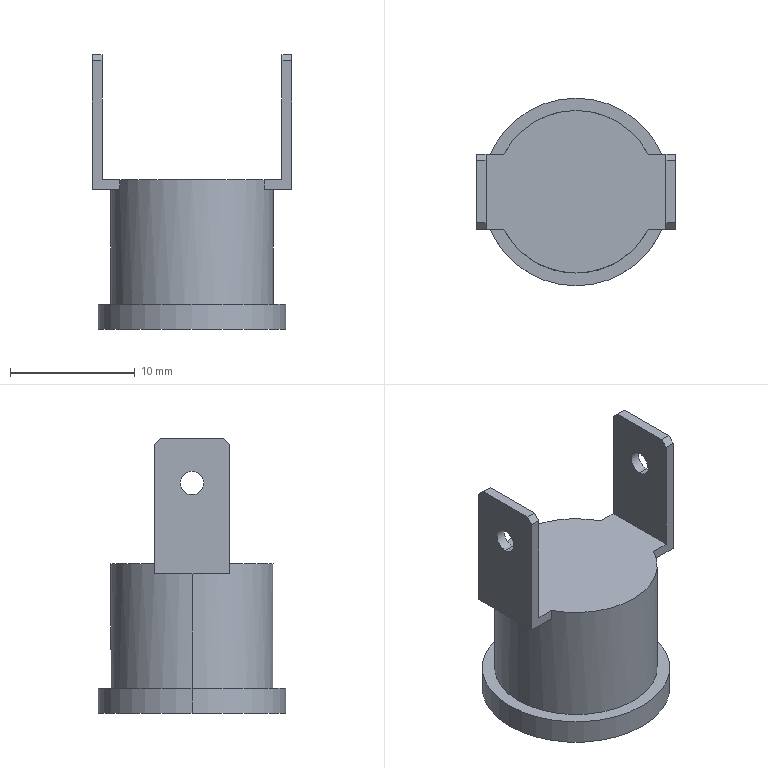Part | STEP file | WENKONG1_2_1_1_1 | 1 solid | 27 faces | box 16 x 15 x 22 mm | volume 1789 mm3 | plane 19 | cylinder 8 | commonest cylinder face diameters 1.882 x4 13 x2 15 x2
STEP:
#1=CARTESIAN_POINT('',(0.,0.,0.));
#2=DIRECTION('',(0.,0.,1.));
#3=DIRECTION('',(1.,0.,0.));
#4=AXIS2_PLACEMENT_3D('',#1,#2,#3);
#5=CARTESIAN_POINT('',(-8.,0.,19.375));
#6=VERTEX_POINT('',#5);
#7=CARTESIAN_POINT('',(-7.2,0.,19.375));
#8=VERTEX_POINT('',#7);
#9=CARTESIAN_POINT('',(-8.,0.,19.375));
#10=DIRECTION('',(1.,0.,0.));
#11=VECTOR('',#10,0.8);
#12=LINE('',#9,#11);
#13=EDGE_CURVE('',#6,#8,#12,.T.);
#14=ORIENTED_EDGE('',*,*,#13,.F.);
#15=CARTESIAN_POINT('',(-8.,0.,17.493));
#16=VERTEX_POINT('',#15);
#17=CARTESIAN_POINT('',(-8.,0.,18.434));
#18=DIRECTION('',(-1.,0.,0.));
#19=DIRECTION('',(0.,0.,-1.));
#20=AXIS2_PLACEMENT_3D('',#17,#18,#19);
#21=CIRCLE('',#20,0.941);
#22=EDGE_CURVE('',#16,#6,#21,.T.);
#23=ORIENTED_EDGE('',*,*,#22,.F.);
#24=CARTESIAN_POINT('',(-7.2,0.,17.493));
#25=VERTEX_POINT('',#24);
#26=CARTESIAN_POINT('',(-7.2,0.,17.493));
#27=DIRECTION('',(-1.,0.,0.));
#28=VECTOR('',#27,0.8);
#29=LINE('',#26,#28);
#30=EDGE_CURVE('',#25,#16,#29,.T.);
#31=ORIENTED_EDGE('',*,*,#30,.F.);
#32=CARTESIAN_POINT('',(-7.2,0.,18.434));
#33=DIRECTION('',(1.,0.,0.));
#34=DIRECTION('',(0.,0.,1.));
#35=AXIS2_PLACEMENT_3D('',#32,#33,#34);
#36=CIRCLE('',#35,0.941);
#37=EDGE_CURVE('',#8,#25,#36,.T.);
#38=ORIENTED_EDGE('',*,*,#37,.F.);
#39=EDGE_LOOP('',(#14,#23,#31,#38));
#40=FACE_OUTER_BOUND('',#39,.F.);
#41=CARTESIAN_POINT('',(-7.6,0.,18.434));
#42=DIRECTION('',(-1.,0.,0.));
#43=DIRECTION('',(0.,0.,-1.));
#44=AXIS2_PLACEMENT_3D('',#41,#42,#43);
#45=CYLINDRICAL_SURFACE('',#44,0.941);
#46=ADVANCED_FACE('',(#40),#45,.F.);
#47=CARTESIAN_POINT('',(-8.,0.,18.434));
#48=DIRECTION('',(-1.,0.,0.));
#49=DIRECTION('',(0.,0.,1.));
#50=AXIS2_PLACEMENT_3D('',#47,#48,#49);
#51=CIRCLE('',#50,0.941);
#52=EDGE_CURVE('',#6,#16,#51,.T.);
#53=ORIENTED_EDGE('',*,*,#52,.F.);
#54=ORIENTED_EDGE('',*,*,#13,.T.);
#55=CARTESIAN_POINT('',(-7.2,0.,18.434));
#56=DIRECTION('',(1.,0.,0.));
#57=DIRECTION('',(0.,0.,-1.));
#58=AXIS2_PLACEMENT_3D('',#55,#56,#57);
#59=CIRCLE('',#58,0.941);
#60=EDGE_CURVE('',#25,#8,#59,.T.);
#61=ORIENTED_EDGE('',*,*,#60,.F.);
#62=ORIENTED_EDGE('',*,*,#30,.T.);
#63=EDGE_LOOP('',(#53,#54,#61,#62));
#64=FACE_OUTER_BOUND('',#63,.F.);
#65=CARTESIAN_POINT('',(-7.6,0.,18.434));
#66=DIRECTION('',(-1.,0.,0.));
#67=DIRECTION('',(0.,0.,1.));
#68=AXIS2_PLACEMENT_3D('',#65,#66,#67);
#69=CYLINDRICAL_SURFACE('',#68,0.941);
#70=ADVANCED_FACE('',(#64),#69,.F.);
#71=CARTESIAN_POINT('',(-8.,2.5,22.));
#72=VERTEX_POINT('',#71);
#73=CARTESIAN_POINT('',(-8.,-2.5,22.));
#74=VERTEX_POINT('',#73);
#75=CARTESIAN_POINT('',(-8.,2.5,22.));
#76=DIRECTION('',(0.,-1.,0.));
#77=VECTOR('',#76,5.);
#78=LINE('',#75,#77);
#79=EDGE_CURVE('',#72,#74,#78,.T.);
#80=ORIENTED_EDGE('',*,*,#79,.T.);
#81=CARTESIAN_POINT('',(-8.,-3.,21.5));
#82=VERTEX_POINT('',#81);
#83=CARTESIAN_POINT('',(-8.,-2.5,22.));
#84=DIRECTION('',(0.,-0.7071,-0.7071));
#85=VECTOR('',#84,0.7071);
#86=LINE('',#83,#85);
#87=EDGE_CURVE('',#74,#82,#86,.T.);
#88=ORIENTED_EDGE('',*,*,#87,.T.);
#89=CARTESIAN_POINT('',(-8.,-3.,11.2));
#90=VERTEX_POINT('',#89);
#91=CARTESIAN_POINT('',(-8.,-3.,21.5));
#92=DIRECTION('',(0.,0.,-1.));
#93=VECTOR('',#92,10.3);
#94=LINE('',#91,#93);
#95=EDGE_CURVE('',#82,#90,#94,.T.);
#96=ORIENTED_EDGE('',*,*,#95,.T.);
#97=CARTESIAN_POINT('',(-8.,3.,11.2));
#98=VERTEX_POINT('',#97);
#99=CARTESIAN_POINT('',(-8.,-3.,11.2));
#100=DIRECTION('',(0.,1.,0.));
#101=VECTOR('',#100,6.);
#102=LINE('',#99,#101);
#103=EDGE_CURVE('',#90,#98,#102,.T.);
#104=ORIENTED_EDGE('',*,*,#103,.T.);
#105=CARTESIAN_POINT('',(-8.,3.,21.5));
#106=VERTEX_POINT('',#105);
#107=CARTESIAN_POINT('',(-8.,3.,11.2));
#108=DIRECTION('',(0.,0.,1.));
#109=VECTOR('',#108,10.3);
#110=LINE('',#107,#109);
#111=EDGE_CURVE('',#98,#106,#110,.T.);
#112=ORIENTED_EDGE('',*,*,#111,.T.);
#113=CARTESIAN_POINT('',(-8.,3.,21.5));
#114=DIRECTION('',(0.,-0.7071,0.7071));
#115=VECTOR('',#114,0.7071);
#116=LINE('',#113,#115);
#117=EDGE_CURVE('',#106,#72,#116,.T.);
#118=ORIENTED_EDGE('',*,*,#117,.T.);
#119=EDGE_LOOP('',(#80,#88,#96,#104,#112,#118));
#120=FACE_OUTER_BOUND('',#119,.F.);
#121=ORIENTED_EDGE('',*,*,#52,.T.);
#122=ORIENTED_EDGE('',*,*,#22,.T.);
#123=EDGE_LOOP('',(#121,#122));
#124=FACE_BOUND('',#123,.F.);
#125=CARTESIAN_POINT('',(-8.,0.,16.6));
#126=DIRECTION('',(1.,0.,0.));
#127=DIRECTION('',(0.,0.,1.));
#128=AXIS2_PLACEMENT_3D('',#125,#126,#127);
#129=PLANE('',#128);
#130=ADVANCED_FACE('',(#120,#124),#129,.F.);
#131=CARTESIAN_POINT('',(-7.2,-2.5,22.));
#132=VERTEX_POINT('',#131);
#133=CARTESIAN_POINT('',(-7.2,2.5,22.));
#134=VERTEX_POINT('',#133);
#135=CARTESIAN_POINT('',(-7.2,-2.5,22.));
#136=DIRECTION('',(0.,1.,0.));
#137=VECTOR('',#136,5.);
#138=LINE('',#135,#137);
#139=EDGE_CURVE('',#132,#134,#138,.T.);
#140=ORIENTED_EDGE('',*,*,#139,.F.);
#141=CARTESIAN_POINT('',(-8.,-2.5,22.));
#142=DIRECTION('',(1.,0.,0.));
#143=VECTOR('',#142,0.8);
#144=LINE('',#141,#143);
#145=EDGE_CURVE('',#74,#132,#144,.T.);
#146=ORIENTED_EDGE('',*,*,#145,.F.);
#147=ORIENTED_EDGE('',*,*,#79,.F.);
#148=CARTESIAN_POINT('',(-7.2,2.5,22.));
#149=DIRECTION('',(-1.,0.,0.));
#150=VECTOR('',#149,0.8);
#151=LINE('',#148,#150);
#152=EDGE_CURVE('',#134,#72,#151,.T.);
#153=ORIENTED_EDGE('',*,*,#152,.F.);
#154=EDGE_LOOP('',(#140,#146,#147,#153));
#155=FACE_OUTER_BOUND('',#154,.F.);
#156=CARTESIAN_POINT('',(-7.6,0.,22.));
#157=DIRECTION('',(0.,0.,1.));
#158=DIRECTION('',(1.,0.,0.));
#159=AXIS2_PLACEMENT_3D('',#156,#157,#158);
#160=PLANE('',#159);
#161=ADVANCED_FACE('',(#155),#160,.T.);
#162=CARTESIAN_POINT('',(-7.2,3.,12.));
#163=VERTEX_POINT('',#162);
#164=CARTESIAN_POINT('',(-7.2,-3.,12.));
#165=VERTEX_POINT('',#164);
#166=CARTESIAN_POINT('',(-7.2,3.,12.));
#167=DIRECTION('',(0.,-1.,0.));
#168=VECTOR('',#167,6.);
#169=LINE('',#166,#168);
#170=EDGE_CURVE('',#163,#165,#169,.T.);
#171=ORIENTED_EDGE('',*,*,#170,.T.);
#172=CARTESIAN_POINT('',(-7.2,-3.,21.5));
#173=VERTEX_POINT('',#172);
#174=CARTESIAN_POINT('',(-7.2,-3.,12.));
#175=DIRECTION('',(0.,0.,1.));
#176=VECTOR('',#175,9.5);
#177=LINE('',#174,#176);
#178=EDGE_CURVE('',#165,#173,#177,.T.);
#179=ORIENTED_EDGE('',*,*,#178,.T.);
#180=CARTESIAN_POINT('',(-7.2,-3.,21.5));
#181=DIRECTION('',(0.,0.7071,0.7071));
#182=VECTOR('',#181,0.7071);
#183=LINE('',#180,#182);
#184=EDGE_CURVE('',#173,#132,#183,.T.);
#185=ORIENTED_EDGE('',*,*,#184,.T.);
#186=ORIENTED_EDGE('',*,*,#139,.T.);
#187=CARTESIAN_POINT('',(-7.2,3.,21.5));
#188=VERTEX_POINT('',#187);
#189=CARTESIAN_POINT('',(-7.2,2.5,22.));
#190=DIRECTION('',(0.,0.7071,-0.7071));
#191=VECTOR('',#190,0.7071);
#192=LINE('',#189,#191);
#193=EDGE_CURVE('',#134,#188,#192,.T.);
#194=ORIENTED_EDGE('',*,*,#193,.T.);
#195=CARTESIAN_POINT('',(-7.2,3.,21.5));
#196=DIRECTION('',(0.,0.,-1.));
#197=VECTOR('',#196,9.5);
#198=LINE('',#195,#197);
#199=EDGE_CURVE('',#188,#163,#198,.T.);
#200=ORIENTED_EDGE('',*,*,#199,.T.);
#201=EDGE_LOOP('',(#171,#179,#185,#186,#194,#200));
#202=FACE_OUTER_BOUND('',#201,.F.);
#203=ORIENTED_EDGE('',*,*,#37,.T.);
#204=ORIENTED_EDGE('',*,*,#60,.T.);
#205=EDGE_LOOP('',(#203,#204));
#206=FACE_BOUND('',#205,.F.);
#207=CARTESIAN_POINT('',(-7.2,0.,17.));
#208=DIRECTION('',(1.,0.,0.));
#209=DIRECTION('',(0.,-1.,0.));
#210=AXIS2_PLACEMENT_3D('',#207,#208,#209);
#211=PLANE('',#210);
#212=ADVANCED_FACE('',(#202,#206),#211,.T.);
#213=CARTESIAN_POINT('',(7.2,-3.,12.));
#214=VERTEX_POINT('',#213);
#215=CARTESIAN_POINT('',(5.766,-3.,12.));
#216=VERTEX_POINT('',#215);
#217=CARTESIAN_POINT('',(7.2,-3.,12.));
#218=DIRECTION('',(-1.,0.,0.));
#219=VECTOR('',#218,1.434);
#220=LINE('',#217,#219);
#221=EDGE_CURVE('',#214,#216,#220,.T.);
#222=ORIENTED_EDGE('',*,*,#221,.T.);
#223=CARTESIAN_POINT('',(-5.766,-3.,12.));
#224=VERTEX_POINT('',#223);
#225=CARTESIAN_POINT('',(0.,0.,12.));
#226=DIRECTION('',(0.,0.,-1.));
#227=DIRECTION('',(0.8871,-0.4615,0.));
#228=AXIS2_PLACEMENT_3D('',#225,#226,#227);
#229=CIRCLE('',#228,6.5);
#230=EDGE_CURVE('',#216,#224,#229,.T.);
#231=ORIENTED_EDGE('',*,*,#230,.T.);
#232=CARTESIAN_POINT('',(-5.766,-3.,12.));
#233=DIRECTION('',(-1.,0.,0.));
#234=VECTOR('',#233,1.434);
#235=LINE('',#232,#234);
#236=EDGE_CURVE('',#224,#165,#235,.T.);
#237=ORIENTED_EDGE('',*,*,#236,.T.);
#238=ORIENTED_EDGE('',*,*,#170,.F.);
#239=CARTESIAN_POINT('',(-5.766,3.,12.));
#240=VERTEX_POINT('',#239);
#241=CARTESIAN_POINT('',(-7.2,3.,12.));
#242=DIRECTION('',(1.,0.,0.));
#243=VECTOR('',#242,1.434);
#244=LINE('',#241,#243);
#245=EDGE_CURVE('',#163,#240,#244,.T.);
#246=ORIENTED_EDGE('',*,*,#245,.T.);
#247=CARTESIAN_POINT('',(5.766,3.,12.));
#248=VERTEX_POINT('',#247);
#249=CARTESIAN_POINT('',(0.,0.,12.));
#250=DIRECTION('',(0.,0.,-1.));
#251=DIRECTION('',(-0.8871,0.4615,0.));
#252=AXIS2_PLACEMENT_3D('',#249,#250,#251);
#253=CIRCLE('',#252,6.5);
#254=EDGE_CURVE('',#240,#248,#253,.T.);
#255=ORIENTED_EDGE('',*,*,#254,.T.);
#256=CARTESIAN_POINT('',(7.2,3.,12.));
#257=VERTEX_POINT('',#256);
#258=CARTESIAN_POINT('',(5.766,3.,12.));
#259=DIRECTION('',(1.,0.,0.));
#260=VECTOR('',#259,1.434);
#261=LINE('',#258,#260);
#262=EDGE_CURVE('',#248,#257,#261,.T.);
#263=ORIENTED_EDGE('',*,*,#262,.T.);
#264=CARTESIAN_POINT('',(7.2,-3.,12.));
#265=DIRECTION('',(0.,1.,0.));
#266=VECTOR('',#265,6.);
#267=LINE('',#264,#266);
#268=EDGE_CURVE('',#214,#257,#267,.T.);
#269=ORIENTED_EDGE('',*,*,#268,.F.);
#270=EDGE_LOOP('',(#222,#231,#237,#238,#246,#255,#263,#269));
#271=FACE_OUTER_BOUND('',#270,.F.);
#272=CARTESIAN_POINT('',(0.,0.,12.));
#273=DIRECTION('',(0.,0.,1.));
#274=DIRECTION('',(1.,0.,0.));
#275=AXIS2_PLACEMENT_3D('',#272,#273,#274);
#276=PLANE('',#275);
#277=ADVANCED_FACE('',(#271),#276,.T.);
#278=CARTESIAN_POINT('',(8.,-3.,21.5));
#279=VERTEX_POINT('',#278);
#280=CARTESIAN_POINT('',(8.,-3.,11.2));
#281=VERTEX_POINT('',#280);
#282=CARTESIAN_POINT('',(8.,-3.,21.5));
#283=DIRECTION('',(0.,0.,-1.));
#284=VECTOR('',#283,10.3);
#285=LINE('',#282,#284);
#286=EDGE_CURVE('',#279,#281,#285,.T.);
#287=ORIENTED_EDGE('',*,*,#286,.T.);
#288=CARTESIAN_POINT('',(5.766,-3.,11.2));
#289=VERTEX_POINT('',#288);
#290=CARTESIAN_POINT('',(5.766,-3.,11.2));
#291=DIRECTION('',(1.,0.,0.));
#292=VECTOR('',#291,2.234);
#293=LINE('',#290,#292);
#294=EDGE_CURVE('',#289,#281,#293,.T.);
#295=ORIENTED_EDGE('',*,*,#294,.F.);
#296=CARTESIAN_POINT('',(5.766,-3.,12.));
#297=DIRECTION('',(0.,0.,-1.));
#298=VECTOR('',#297,0.8);
#299=LINE('',#296,#298);
#300=EDGE_CURVE('',#216,#289,#299,.T.);
#301=ORIENTED_EDGE('',*,*,#300,.F.);
#302=ORIENTED_EDGE('',*,*,#221,.F.);
#303=CARTESIAN_POINT('',(7.2,-3.,21.5));
#304=VERTEX_POINT('',#303);
#305=CARTESIAN_POINT('',(7.2,-3.,21.5));
#306=DIRECTION('',(0.,0.,-1.));
#307=VECTOR('',#306,9.5);
#308=LINE('',#305,#307);
#309=EDGE_CURVE('',#304,#214,#308,.T.);
#310=ORIENTED_EDGE('',*,*,#309,.F.);
#311=CARTESIAN_POINT('',(8.,-3.,21.5));
#312=DIRECTION('',(-1.,0.,0.));
#313=VECTOR('',#312,0.8);
#314=LINE('',#311,#313);
#315=EDGE_CURVE('',#279,#304,#314,.T.);
#316=ORIENTED_EDGE('',*,*,#315,.F.);
#317=EDGE_LOOP('',(#287,#295,#301,#302,#310,#316));
#318=FACE_OUTER_BOUND('',#317,.F.);
#319=CARTESIAN_POINT('',(6.883,-3.,16.35));
#320=DIRECTION('',(0.,1.,0.));
#321=DIRECTION('',(0.,0.,-1.));
#322=AXIS2_PLACEMENT_3D('',#319,#320,#321);
#323=PLANE('',#322);
#324=ADVANCED_FACE('',(#318),#323,.F.);
#325=CARTESIAN_POINT('',(8.,-2.5,22.));
#326=VERTEX_POINT('',#325);
#327=CARTESIAN_POINT('',(8.,2.5,22.));
#328=VERTEX_POINT('',#327);
#329=CARTESIAN_POINT('',(8.,-2.5,22.));
#330=DIRECTION('',(0.,1.,0.));
#331=VECTOR('',#330,5.);
#332=LINE('',#329,#331);
#333=EDGE_CURVE('',#326,#328,#332,.T.);
#334=ORIENTED_EDGE('',*,*,#333,.T.);
#335=CARTESIAN_POINT('',(8.,3.,21.5));
#336=VERTEX_POINT('',#335);
#337=CARTESIAN_POINT('',(8.,2.5,22.));
#338=DIRECTION('',(0.,0.7071,-0.7071));
#339=VECTOR('',#338,0.7071);
#340=LINE('',#337,#339);
#341=EDGE_CURVE('',#328,#336,#340,.T.);
#342=ORIENTED_EDGE('',*,*,#341,.T.);
#343=CARTESIAN_POINT('',(8.,3.,11.2));
#344=VERTEX_POINT('',#343);
#345=CARTESIAN_POINT('',(8.,3.,11.2));
#346=DIRECTION('',(0.,0.,1.));
#347=VECTOR('',#346,10.3);
#348=LINE('',#345,#347);
#349=EDGE_CURVE('',#344,#336,#348,.T.);
#350=ORIENTED_EDGE('',*,*,#349,.F.);
#351=CARTESIAN_POINT('',(8.,-3.,11.2));
#352=DIRECTION('',(0.,1.,0.));
#353=VECTOR('',#352,6.);
#354=LINE('',#351,#353);
#355=EDGE_CURVE('',#281,#344,#354,.T.);
#356=ORIENTED_EDGE('',*,*,#355,.F.);
#357=ORIENTED_EDGE('',*,*,#286,.F.);
#358=CARTESIAN_POINT('',(8.,-3.,21.5));
#359=DIRECTION('',(0.,0.7071,0.7071));
#360=VECTOR('',#359,0.7071);
#361=LINE('',#358,#360);
#362=EDGE_CURVE('',#279,#326,#361,.T.);
#363=ORIENTED_EDGE('',*,*,#362,.T.);
#364=EDGE_LOOP('',(#334,#342,#350,#356,#357,#363));
#365=FACE_OUTER_BOUND('',#364,.F.);
#366=CARTESIAN_POINT('',(8.,0.,19.375));
#367=VERTEX_POINT('',#366);
#368=CARTESIAN_POINT('',(8.,0.,17.493));
#369=VERTEX_POINT('',#368);
#370=CARTESIAN_POINT('',(8.,0.,18.434));
#371=DIRECTION('',(1.,0.,0.));
#372=DIRECTION('',(0.,0.,1.));
#373=AXIS2_PLACEMENT_3D('',#370,#371,#372);
#374=CIRCLE('',#373,0.941);
#375=EDGE_CURVE('',#367,#369,#374,.T.);
#376=ORIENTED_EDGE('',*,*,#375,.T.);
#377=CARTESIAN_POINT('',(8.,0.,18.434));
#378=DIRECTION('',(1.,0.,0.));
#379=DIRECTION('',(0.,0.,-1.));
#380=AXIS2_PLACEMENT_3D('',#377,#378,#379);
#381=CIRCLE('',#380,0.941);
#382=EDGE_CURVE('',#369,#367,#381,.T.);
#383=ORIENTED_EDGE('',*,*,#382,.T.);
#384=EDGE_LOOP('',(#376,#383));
#385=FACE_BOUND('',#384,.F.);
#386=CARTESIAN_POINT('',(8.,0.,16.6));
#387=DIRECTION('',(1.,0.,0.));
#388=DIRECTION('',(0.,0.,-1.));
#389=AXIS2_PLACEMENT_3D('',#386,#387,#388);
#390=PLANE('',#389);
#391=ADVANCED_FACE('',(#365,#385),#390,.T.);
#392=CARTESIAN_POINT('',(7.2,2.5,22.));
#393=VERTEX_POINT('',#392);
#394=CARTESIAN_POINT('',(7.2,-2.5,22.));
#395=VERTEX_POINT('',#394);
#396=CARTESIAN_POINT('',(7.2,2.5,22.));
#397=DIRECTION('',(0.,-1.,0.));
#398=VECTOR('',#397,5.);
#399=LINE('',#396,#398);
#400=EDGE_CURVE('',#393,#395,#399,.T.);
#401=ORIENTED_EDGE('',*,*,#400,.F.);
#402=CARTESIAN_POINT('',(8.,2.5,22.));
#403=DIRECTION('',(-1.,0.,0.));
#404=VECTOR('',#403,0.8);
#405=LINE('',#402,#404);
#406=EDGE_CURVE('',#328,#393,#405,.T.);
#407=ORIENTED_EDGE('',*,*,#406,.F.);
#408=ORIENTED_EDGE('',*,*,#333,.F.);
#409=CARTESIAN_POINT('',(7.2,-2.5,22.));
#410=DIRECTION('',(1.,0.,0.));
#411=VECTOR('',#410,0.8);
#412=LINE('',#409,#411);
#413=EDGE_CURVE('',#395,#326,#412,.T.);
#414=ORIENTED_EDGE('',*,*,#413,.F.);
#415=EDGE_LOOP('',(#401,#407,#408,#414));
#416=FACE_OUTER_BOUND('',#415,.F.);
#417=CARTESIAN_POINT('',(7.6,0.,22.));
#418=DIRECTION('',(0.,0.,1.));
#419=DIRECTION('',(1.,0.,0.));
#420=AXIS2_PLACEMENT_3D('',#417,#418,#419);
#421=PLANE('',#420);
#422=ADVANCED_FACE('',(#416),#421,.T.);
#423=ORIENTED_EDGE('',*,*,#268,.T.);
#424=CARTESIAN_POINT('',(7.2,3.,21.5));
#425=VERTEX_POINT('',#424);
#426=CARTESIAN_POINT('',(7.2,3.,12.));
#427=DIRECTION('',(0.,0.,1.));
#428=VECTOR('',#427,9.5);
#429=LINE('',#426,#428);
#430=EDGE_CURVE('',#257,#425,#429,.T.);
#431=ORIENTED_EDGE('',*,*,#430,.T.);
#432=CARTESIAN_POINT('',(7.2,3.,21.5));
#433=DIRECTION('',(0.,-0.7071,0.7071));
#434=VECTOR('',#433,0.7071);
#435=LINE('',#432,#434);
#436=EDGE_CURVE('',#425,#393,#435,.T.);
#437=ORIENTED_EDGE('',*,*,#436,.T.);
#438=ORIENTED_EDGE('',*,*,#400,.T.);
#439=CARTESIAN_POINT('',(7.2,-2.5,22.));
#440=DIRECTION('',(0.,-0.7071,-0.7071));
#441=VECTOR('',#440,0.7071);
#442=LINE('',#439,#441);
#443=EDGE_CURVE('',#395,#304,#442,.T.);
#444=ORIENTED_EDGE('',*,*,#443,.T.);
#445=ORIENTED_EDGE('',*,*,#309,.T.);
#446=EDGE_LOOP('',(#423,#431,#437,#438,#444,#445));
#447=FACE_OUTER_BOUND('',#446,.F.);
#448=CARTESIAN_POINT('',(7.2,0.,19.375));
#449=VERTEX_POINT('',#448);
#450=CARTESIAN_POINT('',(7.2,0.,17.493));
#451=VERTEX_POINT('',#450);
#452=CARTESIAN_POINT('',(7.2,0.,18.434));
#453=DIRECTION('',(-1.,0.,0.));
#454=DIRECTION('',(0.,0.,1.));
#455=AXIS2_PLACEMENT_3D('',#452,#453,#454);
#456=CIRCLE('',#455,0.941);
#457=EDGE_CURVE('',#449,#451,#456,.T.);
#458=ORIENTED_EDGE('',*,*,#457,.T.);
#459=CARTESIAN_POINT('',(7.2,0.,18.434));
#460=DIRECTION('',(-1.,0.,0.));
#461=DIRECTION('',(0.,0.,-1.));
#462=AXIS2_PLACEMENT_3D('',#459,#460,#461);
#463=CIRCLE('',#462,0.941);
#464=EDGE_CURVE('',#451,#449,#463,.T.);
#465=ORIENTED_EDGE('',*,*,#464,.T.);
#466=EDGE_LOOP('',(#458,#465));
#467=FACE_BOUND('',#466,.F.);
#468=CARTESIAN_POINT('',(7.2,0.,17.));
#469=DIRECTION('',(1.,0.,0.));
#470=DIRECTION('',(0.,1.,0.));
#471=AXIS2_PLACEMENT_3D('',#468,#469,#470);
#472=PLANE('',#471);
#473=ADVANCED_FACE('',(#447,#467),#472,.F.);
#474=ORIENTED_EDGE('',*,*,#430,.F.);
#475=ORIENTED_EDGE('',*,*,#262,.F.);
#476=CARTESIAN_POINT('',(5.766,3.,11.2));
#477=VERTEX_POINT('',#476);
#478=CARTESIAN_POINT('',(5.766,3.,11.2));
#479=DIRECTION('',(0.,0.,1.));
#480=VECTOR('',#479,0.8);
#481=LINE('',#478,#480);
#482=EDGE_CURVE('',#477,#248,#481,.T.);
#483=ORIENTED_EDGE('',*,*,#482,.F.);
#484=CARTESIAN_POINT('',(8.,3.,11.2));
#485=DIRECTION('',(-1.,0.,0.));
#486=VECTOR('',#485,2.234);
#487=LINE('',#484,#486);
#488=EDGE_CURVE('',#344,#477,#487,.T.);
#489=ORIENTED_EDGE('',*,*,#488,.F.);
#490=ORIENTED_EDGE('',*,*,#349,.T.);
#491=CARTESIAN_POINT('',(7.2,3.,21.5));
#492=DIRECTION('',(1.,0.,0.));
#493=VECTOR('',#492,0.8);
#494=LINE('',#491,#493);
#495=EDGE_CURVE('',#425,#336,#494,.T.);
#496=ORIENTED_EDGE('',*,*,#495,.F.);
#497=EDGE_LOOP('',(#474,#475,#483,#489,#490,#496));
#498=FACE_OUTER_BOUND('',#497,.F.);
#499=CARTESIAN_POINT('',(6.883,3.,16.35));
#500=DIRECTION('',(0.,1.,0.));
#501=DIRECTION('',(0.,0.,1.));
#502=AXIS2_PLACEMENT_3D('',#499,#500,#501);
#503=PLANE('',#502);
#504=ADVANCED_FACE('',(#498),#503,.T.);
#505=CARTESIAN_POINT('',(6.5,0.000000002,11.2));
#506=VERTEX_POINT('',#505);
#507=CARTESIAN_POINT('',(0.,0.,11.2));
#508=DIRECTION('',(0.,0.,-1.));
#509=DIRECTION('',(0.8871,0.4615,0.));
#510=AXIS2_PLACEMENT_3D('',#507,#508,#509);
#511=CIRCLE('',#510,6.5);
#512=EDGE_CURVE('',#477,#506,#511,.T.);
#513=ORIENTED_EDGE('',*,*,#512,.F.);
#514=ORIENTED_EDGE('',*,*,#482,.T.);
#515=ORIENTED_EDGE('',*,*,#254,.F.);
#516=CARTESIAN_POINT('',(-5.766,3.,11.2));
#517=VERTEX_POINT('',#516);
#518=CARTESIAN_POINT('',(-5.766,3.,12.));
#519=DIRECTION('',(0.,0.,-1.));
#520=VECTOR('',#519,0.8);
#521=LINE('',#518,#520);
#522=EDGE_CURVE('',#240,#517,#521,.T.);
#523=ORIENTED_EDGE('',*,*,#522,.T.);
#524=CARTESIAN_POINT('',(-6.5,-0.000000002,11.2));
#525=VERTEX_POINT('',#524);
#526=CARTESIAN_POINT('',(0.,0.,11.2));
#527=DIRECTION('',(0.,0.,-1.));
#528=DIRECTION('',(-1.,0.,0.));
#529=AXIS2_PLACEMENT_3D('',#526,#527,#528);
#530=CIRCLE('',#529,6.5);
#531=EDGE_CURVE('',#525,#517,#530,.T.);
#532=ORIENTED_EDGE('',*,*,#531,.F.);
#533=CARTESIAN_POINT('',(-6.5,0.,2.));
#534=VERTEX_POINT('',#533);
#535=CARTESIAN_POINT('',(-6.5,-0.000000001,11.2));
#536=DIRECTION('',(0.,0.,-1.));
#537=VECTOR('',#536,9.2);
#538=LINE('',#535,#537);
#539=EDGE_CURVE('',#525,#534,#538,.T.);
#540=ORIENTED_EDGE('',*,*,#539,.T.);
#541=CARTESIAN_POINT('',(6.5,0.,2.));
#542=VERTEX_POINT('',#541);
#543=CARTESIAN_POINT('',(0.,0.,2.));
#544=DIRECTION('',(0.,0.,1.));
#545=DIRECTION('',(1.,0.,0.));
#546=AXIS2_PLACEMENT_3D('',#543,#544,#545);
#547=CIRCLE('',#546,6.5);
#548=EDGE_CURVE('',#542,#534,#547,.T.);
#549=ORIENTED_EDGE('',*,*,#548,.F.);
#550=CARTESIAN_POINT('',(6.5,0.,2.));
#551=DIRECTION('',(0.,0.,1.));
#552=VECTOR('',#551,9.2);
#553=LINE('',#550,#552);
#554=EDGE_CURVE('',#542,#506,#553,.T.);
#555=ORIENTED_EDGE('',*,*,#554,.T.);
#556=EDGE_LOOP('',(#513,#514,#515,#523,#532,#540,#549,#555));
#557=FACE_OUTER_BOUND('',#556,.F.);
#558=CARTESIAN_POINT('',(0.,0.,7.));
#559=DIRECTION('',(0.,0.,-1.));
#560=DIRECTION('',(-1.,0.,0.));
#561=AXIS2_PLACEMENT_3D('',#558,#559,#560);
#562=CYLINDRICAL_SURFACE('',#561,6.5);
#563=ADVANCED_FACE('',(#557),#562,.T.);
#564=ORIENTED_EDGE('',*,*,#512,.T.);
#565=CARTESIAN_POINT('',(0.,0.,11.2));
#566=DIRECTION('',(0.,0.,-1.));
#567=DIRECTION('',(1.,0.,0.));
#568=AXIS2_PLACEMENT_3D('',#565,#566,#567);
#569=CIRCLE('',#568,6.5);
#570=EDGE_CURVE('',#506,#289,#569,.T.);
#571=ORIENTED_EDGE('',*,*,#570,.T.);
#572=ORIENTED_EDGE('',*,*,#294,.T.);
#573=ORIENTED_EDGE('',*,*,#355,.T.);
#574=ORIENTED_EDGE('',*,*,#488,.T.);
#575=EDGE_LOOP('',(#564,#571,#572,#573,#574));
#576=FACE_OUTER_BOUND('',#575,.F.);
#577=CARTESIAN_POINT('',(6.883,0.,11.2));
#578=DIRECTION('',(0.,0.,1.));
#579=DIRECTION('',(-1.,0.,0.));
#580=AXIS2_PLACEMENT_3D('',#577,#578,#579);
#581=PLANE('',#580);
#582=ADVANCED_FACE('',(#576),#581,.F.);
#583=ORIENTED_EDGE('',*,*,#554,.F.);
#584=CARTESIAN_POINT('',(0.,0.,2.));
#585=DIRECTION('',(0.,0.,1.));
#586=DIRECTION('',(-1.,0.,0.));
#587=AXIS2_PLACEMENT_3D('',#584,#585,#586);
#588=CIRCLE('',#587,6.5);
#589=EDGE_CURVE('',#534,#542,#588,.T.);
#590=ORIENTED_EDGE('',*,*,#589,.F.);
#591=ORIENTED_EDGE('',*,*,#539,.F.);
#592=CARTESIAN_POINT('',(-5.766,-3.,11.2));
#593=VERTEX_POINT('',#592);
#594=CARTESIAN_POINT('',(0.,0.,11.2));
#595=DIRECTION('',(0.,0.,-1.));
#596=DIRECTION('',(-0.8871,-0.4615,0.));
#597=AXIS2_PLACEMENT_3D('',#594,#595,#596);
#598=CIRCLE('',#597,6.5);
#599=EDGE_CURVE('',#593,#525,#598,.T.);
#600=ORIENTED_EDGE('',*,*,#599,.F.);
#601=CARTESIAN_POINT('',(-5.766,-3.,11.2));
#602=DIRECTION('',(0.,0.,1.));
#603=VECTOR('',#602,0.8);
#604=LINE('',#601,#603);
#605=EDGE_CURVE('',#593,#224,#604,.T.);
#606=ORIENTED_EDGE('',*,*,#605,.T.);
#607=ORIENTED_EDGE('',*,*,#230,.F.);
#608=ORIENTED_EDGE('',*,*,#300,.T.);
#609=ORIENTED_EDGE('',*,*,#570,.F.);
#610=EDGE_LOOP('',(#583,#590,#591,#600,#606,#607,#608,#609));
#611=FACE_OUTER_BOUND('',#610,.F.);
#612=CARTESIAN_POINT('',(0.,0.,7.));
#613=DIRECTION('',(0.,0.,-1.));
#614=DIRECTION('',(1.,0.,0.));
#615=AXIS2_PLACEMENT_3D('',#612,#613,#614);
#616=CYLINDRICAL_SURFACE('',#615,6.5);
#617=ADVANCED_FACE('',(#611),#616,.T.);
#618=CARTESIAN_POINT('',(7.5,0.,2.));
#619=VERTEX_POINT('',#618);
#620=CARTESIAN_POINT('',(-7.5,0.,2.));
#621=VERTEX_POINT('',#620);
#622=CARTESIAN_POINT('',(0.,0.,2.));
#623=DIRECTION('',(0.,0.,-1.));
#624=DIRECTION('',(1.,0.,0.));
#625=AXIS2_PLACEMENT_3D('',#622,#623,#624);
#626=CIRCLE('',#625,7.5);
#627=EDGE_CURVE('',#619,#621,#626,.T.);
#628=ORIENTED_EDGE('',*,*,#627,.T.);
#629=CARTESIAN_POINT('',(0.,0.,2.));
#630=DIRECTION('',(0.,0.,-1.));
#631=DIRECTION('',(-1.,0.,0.));
#632=AXIS2_PLACEMENT_3D('',#629,#630,#631);
#633=CIRCLE('',#632,7.5);
#634=EDGE_CURVE('',#621,#619,#633,.T.);
#635=ORIENTED_EDGE('',*,*,#634,.T.);
#636=EDGE_LOOP('',(#628,#635));
#637=FACE_OUTER_BOUND('',#636,.F.);
#638=ORIENTED_EDGE('',*,*,#589,.T.);
#639=ORIENTED_EDGE('',*,*,#548,.T.);
#640=EDGE_LOOP('',(#638,#639));
#641=FACE_BOUND('',#640,.F.);
#642=CARTESIAN_POINT('',(0.,0.,2.));
#643=DIRECTION('',(0.,0.,1.));
#644=DIRECTION('',(1.,0.,0.));
#645=AXIS2_PLACEMENT_3D('',#642,#643,#644);
#646=PLANE('',#645);
#647=ADVANCED_FACE('',(#637,#641),#646,.T.);
#648=CARTESIAN_POINT('',(7.5,0.,0.));
#649=VERTEX_POINT('',#648);
#650=CARTESIAN_POINT('',(7.5,0.,0.));
#651=DIRECTION('',(0.,0.,1.));
#652=VECTOR('',#651,2.);
#653=LINE('',#650,#652);
#654=EDGE_CURVE('',#649,#619,#653,.T.);
#655=ORIENTED_EDGE('',*,*,#654,.F.);
#656=CARTESIAN_POINT('',(-7.5,0.,0.));
#657=VERTEX_POINT('',#656);
#658=CARTESIAN_POINT('',(0.,0.,0.));
#659=DIRECTION('',(0.,0.,1.));
#660=DIRECTION('',(-1.,0.,0.));
#661=AXIS2_PLACEMENT_3D('',#658,#659,#660);
#662=CIRCLE('',#661,7.5);
#663=EDGE_CURVE('',#657,#649,#662,.T.);
#664=ORIENTED_EDGE('',*,*,#663,.F.);
#665=CARTESIAN_POINT('',(-7.5,0.,2.));
#666=DIRECTION('',(0.,0.,-1.));
#667=VECTOR('',#666,2.);
#668=LINE('',#665,#667);
#669=EDGE_CURVE('',#621,#657,#668,.T.);
#670=ORIENTED_EDGE('',*,*,#669,.F.);
#671=ORIENTED_EDGE('',*,*,#627,.F.);
#672=EDGE_LOOP('',(#655,#664,#670,#671));
#673=FACE_OUTER_BOUND('',#672,.F.);
#674=CARTESIAN_POINT('',(0.,0.,1.));
#675=DIRECTION('',(0.,0.,-1.));
#676=DIRECTION('',(1.,0.,0.));
#677=AXIS2_PLACEMENT_3D('',#674,#675,#676);
#678=CYLINDRICAL_SURFACE('',#677,7.5);
#679=ADVANCED_FACE('',(#673),#678,.T.);
#680=ORIENTED_EDGE('',*,*,#634,.F.);
#681=ORIENTED_EDGE('',*,*,#669,.T.);
#682=CARTESIAN_POINT('',(0.,0.,0.));
#683=DIRECTION('',(0.,0.,1.));
#684=DIRECTION('',(1.,0.,0.));
#685=AXIS2_PLACEMENT_3D('',#682,#683,#684);
#686=CIRCLE('',#685,7.5);
#687=EDGE_CURVE('',#649,#657,#686,.T.);
#688=ORIENTED_EDGE('',*,*,#687,.F.);
#689=ORIENTED_EDGE('',*,*,#654,.T.);
#690=EDGE_LOOP('',(#680,#681,#688,#689));
#691=FACE_OUTER_BOUND('',#690,.F.);
#692=CARTESIAN_POINT('',(0.,0.,1.));
#693=DIRECTION('',(0.,0.,-1.));
#694=DIRECTION('',(-1.,0.,0.));
#695=AXIS2_PLACEMENT_3D('',#692,#693,#694);
#696=CYLINDRICAL_SURFACE('',#695,7.5);
#697=ADVANCED_FACE('',(#691),#696,.T.);
#698=ORIENTED_EDGE('',*,*,#687,.T.);
#699=ORIENTED_EDGE('',*,*,#663,.T.);
#700=EDGE_LOOP('',(#698,#699));
#701=FACE_OUTER_BOUND('',#700,.F.);
#702=CARTESIAN_POINT('',(0.,0.,0.));
#703=DIRECTION('',(0.,0.,1.));
#704=DIRECTION('',(1.,0.,0.));
#705=AXIS2_PLACEMENT_3D('',#702,#703,#704);
#706=PLANE('',#705);
#707=ADVANCED_FACE('',(#701),#706,.F.);
#708=ORIENTED_EDGE('',*,*,#599,.T.);
#709=ORIENTED_EDGE('',*,*,#531,.T.);
#710=CARTESIAN_POINT('',(-5.766,3.,11.2));
#711=DIRECTION('',(-1.,0.,0.));
#712=VECTOR('',#711,2.234);
#713=LINE('',#710,#712);
#714=EDGE_CURVE('',#517,#98,#713,.T.);
#715=ORIENTED_EDGE('',*,*,#714,.T.);
#716=ORIENTED_EDGE('',*,*,#103,.F.);
#717=CARTESIAN_POINT('',(-8.,-3.,11.2));
#718=DIRECTION('',(1.,0.,0.));
#719=VECTOR('',#718,2.234);
#720=LINE('',#717,#719);
#721=EDGE_CURVE('',#90,#593,#720,.T.);
#722=ORIENTED_EDGE('',*,*,#721,.T.);
#723=EDGE_LOOP('',(#708,#709,#715,#716,#722));
#724=FACE_OUTER_BOUND('',#723,.F.);
#725=CARTESIAN_POINT('',(-6.883,0.,11.2));
#726=DIRECTION('',(0.,0.,1.));
#727=DIRECTION('',(-1.,0.,0.));
#728=AXIS2_PLACEMENT_3D('',#725,#726,#727);
#729=PLANE('',#728);
#730=ADVANCED_FACE('',(#724),#729,.F.);
#731=ORIENTED_EDGE('',*,*,#111,.F.);
#732=ORIENTED_EDGE('',*,*,#714,.F.);
#733=ORIENTED_EDGE('',*,*,#522,.F.);
#734=ORIENTED_EDGE('',*,*,#245,.F.);
#735=ORIENTED_EDGE('',*,*,#199,.F.);
#736=CARTESIAN_POINT('',(-8.,3.,21.5));
#737=DIRECTION('',(1.,0.,0.));
#738=VECTOR('',#737,0.8);
#739=LINE('',#736,#738);
#740=EDGE_CURVE('',#106,#188,#739,.T.);
#741=ORIENTED_EDGE('',*,*,#740,.F.);
#742=EDGE_LOOP('',(#731,#732,#733,#734,#735,#741));
#743=FACE_OUTER_BOUND('',#742,.F.);
#744=CARTESIAN_POINT('',(-6.883,3.,16.35));
#745=DIRECTION('',(0.,1.,0.));
#746=DIRECTION('',(0.,0.,1.));
#747=AXIS2_PLACEMENT_3D('',#744,#745,#746);
#748=PLANE('',#747);
#749=ADVANCED_FACE('',(#743),#748,.T.);
#750=ORIENTED_EDGE('',*,*,#152,.T.);
#751=ORIENTED_EDGE('',*,*,#117,.F.);
#752=ORIENTED_EDGE('',*,*,#740,.T.);
#753=ORIENTED_EDGE('',*,*,#193,.F.);
#754=EDGE_LOOP('',(#750,#751,#752,#753));
#755=FACE_OUTER_BOUND('',#754,.F.);
#756=CARTESIAN_POINT('',(-7.6,2.75,21.75));
#757=DIRECTION('',(0.,0.7071,0.7071));
#758=DIRECTION('',(-1.,0.,0.));
#759=AXIS2_PLACEMENT_3D('',#756,#757,#758);
#760=PLANE('',#759);
#761=ADVANCED_FACE('',(#755),#760,.T.);
#762=ORIENTED_EDGE('',*,*,#178,.F.);
#763=ORIENTED_EDGE('',*,*,#236,.F.);
#764=ORIENTED_EDGE('',*,*,#605,.F.);
#765=ORIENTED_EDGE('',*,*,#721,.F.);
#766=ORIENTED_EDGE('',*,*,#95,.F.);
#767=CARTESIAN_POINT('',(-7.2,-3.,21.5));
#768=DIRECTION('',(-1.,0.,0.));
#769=VECTOR('',#768,0.8);
#770=LINE('',#767,#769);
#771=EDGE_CURVE('',#173,#82,#770,.T.);
#772=ORIENTED_EDGE('',*,*,#771,.F.);
#773=EDGE_LOOP('',(#762,#763,#764,#765,#766,#772));
#774=FACE_OUTER_BOUND('',#773,.F.);
#775=CARTESIAN_POINT('',(-6.883,-3.,16.35));
#776=DIRECTION('',(0.,1.,0.));
#777=DIRECTION('',(0.,0.,-1.));
#778=AXIS2_PLACEMENT_3D('',#775,#776,#777);
#779=PLANE('',#778);
#780=ADVANCED_FACE('',(#774),#779,.F.);
#781=ORIENTED_EDGE('',*,*,#145,.T.);
#782=ORIENTED_EDGE('',*,*,#184,.F.);
#783=ORIENTED_EDGE('',*,*,#771,.T.);
#784=ORIENTED_EDGE('',*,*,#87,.F.);
#785=EDGE_LOOP('',(#781,#782,#783,#784));
#786=FACE_OUTER_BOUND('',#785,.F.);
#787=CARTESIAN_POINT('',(-7.6,-2.75,21.75));
#788=DIRECTION('',(0.,0.7071,-0.7071));
#789=DIRECTION('',(1.,0.,0.));
#790=AXIS2_PLACEMENT_3D('',#787,#788,#789);
#791=PLANE('',#790);
#792=ADVANCED_FACE('',(#786),#791,.F.);
#793=ORIENTED_EDGE('',*,*,#406,.T.);
#794=ORIENTED_EDGE('',*,*,#436,.F.);
#795=ORIENTED_EDGE('',*,*,#495,.T.);
#796=ORIENTED_EDGE('',*,*,#341,.F.);
#797=EDGE_LOOP('',(#793,#794,#795,#796));
#798=FACE_OUTER_BOUND('',#797,.F.);
#799=CARTESIAN_POINT('',(7.6,2.75,21.75));
#800=DIRECTION('',(0.,0.7071,0.7071));
#801=DIRECTION('',(-1.,0.,0.));
#802=AXIS2_PLACEMENT_3D('',#799,#800,#801);
#803=PLANE('',#802);
#804=ADVANCED_FACE('',(#798),#803,.T.);
#805=ORIENTED_EDGE('',*,*,#413,.T.);
#806=ORIENTED_EDGE('',*,*,#362,.F.);
#807=ORIENTED_EDGE('',*,*,#315,.T.);
#808=ORIENTED_EDGE('',*,*,#443,.F.);
#809=EDGE_LOOP('',(#805,#806,#807,#808));
#810=FACE_OUTER_BOUND('',#809,.F.);
#811=CARTESIAN_POINT('',(7.6,-2.75,21.75));
#812=DIRECTION('',(0.,0.7071,-0.7071));
#813=DIRECTION('',(1.,0.,0.));
#814=AXIS2_PLACEMENT_3D('',#811,#812,#813);
#815=PLANE('',#814);
#816=ADVANCED_FACE('',(#810),#815,.F.);
#817=ORIENTED_EDGE('',*,*,#457,.F.);
#818=CARTESIAN_POINT('',(7.2,0.,19.375));
#819=DIRECTION('',(1.,0.,0.));
#820=VECTOR('',#819,0.8);
#821=LINE('',#818,#820);
#822=EDGE_CURVE('',#449,#367,#821,.T.);
#823=ORIENTED_EDGE('',*,*,#822,.T.);
#824=ORIENTED_EDGE('',*,*,#382,.F.);
#825=CARTESIAN_POINT('',(8.,0.,17.493));
#826=DIRECTION('',(-1.,0.,0.));
#827=VECTOR('',#826,0.8);
#828=LINE('',#825,#827);
#829=EDGE_CURVE('',#369,#451,#828,.T.);
#830=ORIENTED_EDGE('',*,*,#829,.T.);
#831=EDGE_LOOP('',(#817,#823,#824,#830));
#832=FACE_OUTER_BOUND('',#831,.F.);
#833=CARTESIAN_POINT('',(7.6,0.,18.434));
#834=DIRECTION('',(-1.,0.,0.));
#835=DIRECTION('',(0.,0.,1.));
#836=AXIS2_PLACEMENT_3D('',#833,#834,#835);
#837=CYLINDRICAL_SURFACE('',#836,0.941);
#838=ADVANCED_FACE('',(#832),#837,.F.);
#839=ORIENTED_EDGE('',*,*,#822,.F.);
#840=ORIENTED_EDGE('',*,*,#464,.F.);
#841=ORIENTED_EDGE('',*,*,#829,.F.);
#842=ORIENTED_EDGE('',*,*,#375,.F.);
#843=EDGE_LOOP('',(#839,#840,#841,#842));
#844=FACE_OUTER_BOUND('',#843,.F.);
#845=CARTESIAN_POINT('',(7.6,0.,18.434));
#846=DIRECTION('',(-1.,0.,0.));
#847=DIRECTION('',(0.,0.,-1.));
#848=AXIS2_PLACEMENT_3D('',#845,#846,#847);
#849=CYLINDRICAL_SURFACE('',#848,0.941);
#850=ADVANCED_FACE('',(#844),#849,.F.);
#851=CLOSED_SHELL('',(#46,#70,#130,#161,#212,#277,#324,#391,#422,#473,#504,#563,#582,#617,#647,#679,#697,#707,#730,#749,#761,#780,#792,#804,#816,#838,#850));
#852=MANIFOLD_SOLID_BREP('',#851);
#853=(LENGTH_UNIT()NAMED_UNIT(*)SI_UNIT(.MILLI.,.METRE.));
#854=UNCERTAINTY_MEASURE_WITH_UNIT(LENGTH_MEASURE(0.003107),#853,'','');
#855=(NAMED_UNIT(*)PLANE_ANGLE_UNIT()SI_UNIT($,.RADIAN.));
#856=PLANE_ANGLE_MEASURE_WITH_UNIT(PLANE_ANGLE_MEASURE(0.01745),#855);
#857=(CONVERSION_BASED_UNIT('DEGREE',#856)NAMED_UNIT(*)PLANE_ANGLE_UNIT());
#858=(NAMED_UNIT(*)SI_UNIT($,.STERADIAN.)SOLID_ANGLE_UNIT());
#859=(GEOMETRIC_REPRESENTATION_CONTEXT(3)GLOBAL_UNCERTAINTY_ASSIGNED_CONTEXT((#854))GLOBAL_UNIT_ASSIGNED_CONTEXT((#853,#857,#858))REPRESENTATION_CONTEXT('',''));
#860=ADVANCED_BREP_SHAPE_REPRESENTATION('',(#4,#852),#859);